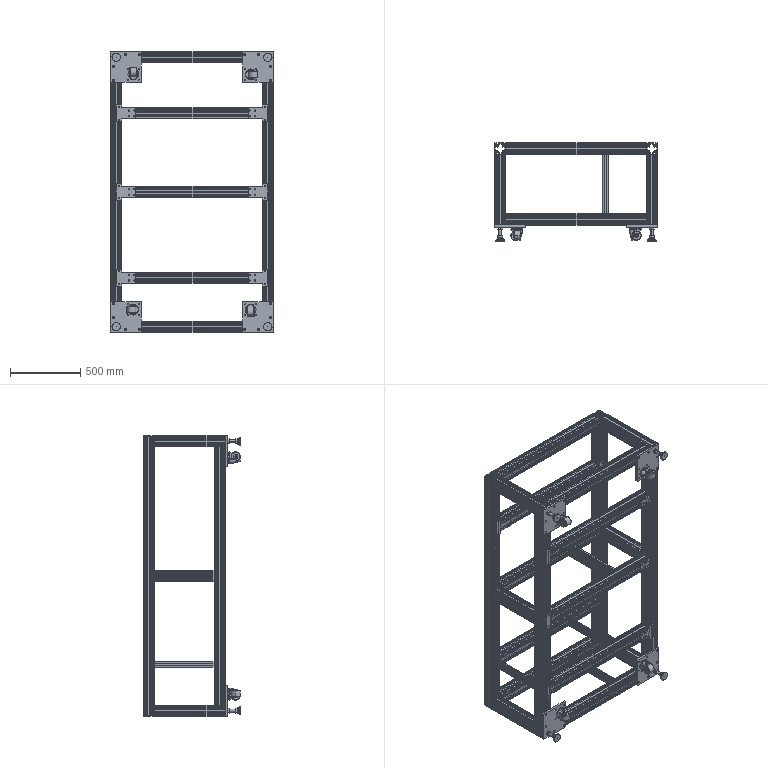Part | SolidWorks | 68 solids | 6018 faces | volume 41198863 mm3 | plane 3698 | cylinder 2048 | cone 152 | torus 104 | sphere 16 | commonest cylinder face diameters 2 x708 0.6 x382 6.8 x272 12 x200 6 x112 9 x96